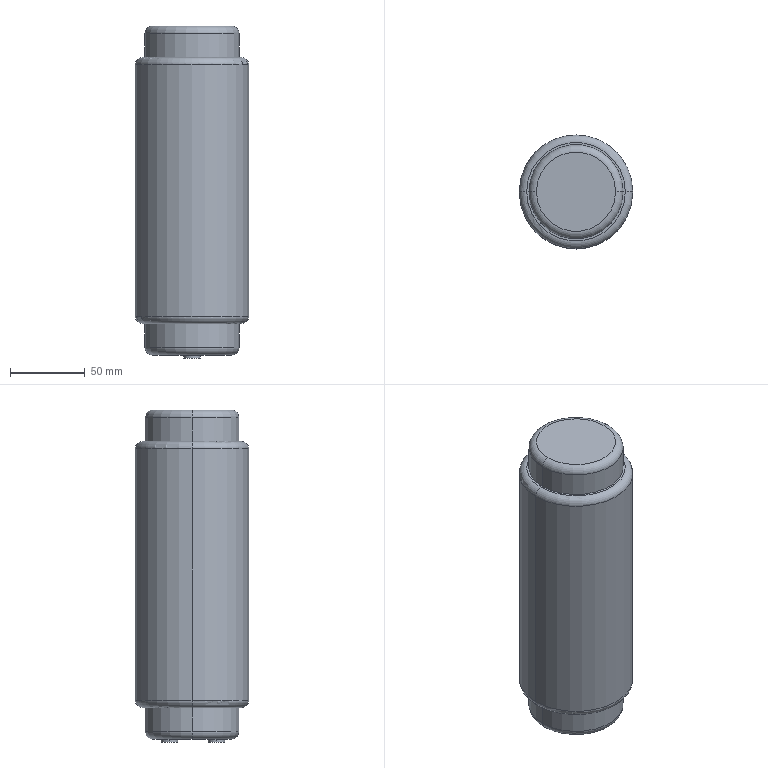Part | SolidWorks | features ICE 3, Extrusion 1, Fillet 1 | 1 solid | 24 faces | box 76 x 76 x 222 mm | volume 934259 mm3 | cylinder 10 | torus 8 | plane 6 | commonest cylinder face diameters 63 x4 10.958 x2 11.023 x2 76 x2
STEP:
#1=CARTESIAN_POINT('',(-5.511,-16.316,-112.));
#2=VERTEX_POINT('',#1);
#3=CARTESIAN_POINT('',(5.511,-16.316,-112.));
#4=VERTEX_POINT('',#3);
#5=CARTESIAN_POINT('',(0.,-16.316,-112.));
#6=DIRECTION('',(0.,0.,-1.));
#7=DIRECTION('',(-1.,0.,0.));
#8=AXIS2_PLACEMENT_3D('',#5,#6,#7);
#9=CIRCLE('',#8,5.511);
#10=EDGE_CURVE('',#2,#4,#9,.T.);
#11=ORIENTED_EDGE('',*,*,#10,.F.);
#12=CARTESIAN_POINT('',(-5.511,-16.316,-110.));
#13=VERTEX_POINT('',#12);
#14=CARTESIAN_POINT('',(-5.511,-16.316,-112.));
#15=DIRECTION('',(0.,0.,1.));
#16=VECTOR('',#15,1000.);
#17=LINE('',#14,#16);
#18=EDGE_CURVE('',#2,#13,#17,.T.);
#19=ORIENTED_EDGE('',*,*,#18,.T.);
#20=CARTESIAN_POINT('',(5.511,-16.316,-110.));
#21=VERTEX_POINT('',#20);
#22=CARTESIAN_POINT('',(0.,-16.316,-110.));
#23=DIRECTION('',(0.,0.,-1.));
#24=DIRECTION('',(1.,0.,0.));
#25=AXIS2_PLACEMENT_3D('',#22,#23,#24);
#26=CIRCLE('',#25,5.511);
#27=EDGE_CURVE('',#13,#21,#26,.T.);
#28=ORIENTED_EDGE('',*,*,#27,.T.);
#29=CARTESIAN_POINT('',(5.511,-16.316,-112.));
#30=DIRECTION('',(0.,0.,1.));
#31=VECTOR('',#30,1000.);
#32=LINE('',#29,#31);
#33=EDGE_CURVE('',#4,#21,#32,.T.);
#34=ORIENTED_EDGE('',*,*,#33,.F.);
#35=EDGE_LOOP('',(#11,#19,#28,#34));
#36=FACE_OUTER_BOUND('',#35,.T.);
#37=CARTESIAN_POINT('',(0.,-16.316,-112.));
#38=DIRECTION('',(0.,0.,1.));
#39=DIRECTION('',(1.,0.,0.));
#40=AXIS2_PLACEMENT_3D('',#37,#38,#39);
#41=CYLINDRICAL_SURFACE('',#40,5.511);
#42=ADVANCED_FACE('',(#36),#41,.T.);
#43=CARTESIAN_POINT('',(-5.479,15.014,-112.));
#44=VERTEX_POINT('',#43);
#45=CARTESIAN_POINT('',(5.479,15.014,-112.));
#46=VERTEX_POINT('',#45);
#47=CARTESIAN_POINT('',(0.,15.014,-112.));
#48=DIRECTION('',(0.,0.,-1.));
#49=DIRECTION('',(-1.,0.,0.));
#50=AXIS2_PLACEMENT_3D('',#47,#48,#49);
#51=CIRCLE('',#50,5.479);
#52=EDGE_CURVE('',#44,#46,#51,.T.);
#53=ORIENTED_EDGE('',*,*,#52,.F.);
#54=CARTESIAN_POINT('',(-5.479,15.014,-110.));
#55=VERTEX_POINT('',#54);
#56=CARTESIAN_POINT('',(-5.479,15.014,-112.));
#57=DIRECTION('',(0.,0.,1.));
#58=VECTOR('',#57,1000.);
#59=LINE('',#56,#58);
#60=EDGE_CURVE('',#44,#55,#59,.T.);
#61=ORIENTED_EDGE('',*,*,#60,.T.);
#62=CARTESIAN_POINT('',(5.479,15.014,-110.));
#63=VERTEX_POINT('',#62);
#64=CARTESIAN_POINT('',(0.,15.014,-110.));
#65=DIRECTION('',(0.,0.,-1.));
#66=DIRECTION('',(1.,0.,0.));
#67=AXIS2_PLACEMENT_3D('',#64,#65,#66);
#68=CIRCLE('',#67,5.479);
#69=EDGE_CURVE('',#55,#63,#68,.T.);
#70=ORIENTED_EDGE('',*,*,#69,.T.);
#71=CARTESIAN_POINT('',(5.479,15.014,-112.));
#72=DIRECTION('',(0.,0.,1.));
#73=VECTOR('',#72,1000.);
#74=LINE('',#71,#73);
#75=EDGE_CURVE('',#46,#63,#74,.T.);
#76=ORIENTED_EDGE('',*,*,#75,.F.);
#77=EDGE_LOOP('',(#53,#61,#70,#76));
#78=FACE_OUTER_BOUND('',#77,.T.);
#79=CARTESIAN_POINT('',(0.,15.014,-112.));
#80=DIRECTION('',(0.,0.,1.));
#81=DIRECTION('',(1.,0.,0.));
#82=AXIS2_PLACEMENT_3D('',#79,#80,#81);
#83=CYLINDRICAL_SURFACE('',#82,5.479);
#84=ADVANCED_FACE('',(#78),#83,.T.);
#85=CARTESIAN_POINT('',(-38.,0.,84.));
#86=VERTEX_POINT('',#85);
#87=CARTESIAN_POINT('',(38.,0.,84.));
#88=VERTEX_POINT('',#87);
#89=CARTESIAN_POINT('',(0.,0.,84.));
#90=DIRECTION('',(0.,0.,-1.));
#91=DIRECTION('',(1.,0.,0.));
#92=AXIS2_PLACEMENT_3D('',#89,#90,#91);
#93=CIRCLE('',#92,38.);
#94=EDGE_CURVE('',#86,#88,#93,.T.);
#95=ORIENTED_EDGE('',*,*,#94,.F.);
#96=CARTESIAN_POINT('',(-33.,0.,89.));
#97=VERTEX_POINT('',#96);
#98=CARTESIAN_POINT('',(-33.,0.,84.));
#99=DIRECTION('',(0.,1.,0.));
#100=DIRECTION('',(-1.,0.,0.));
#101=AXIS2_PLACEMENT_3D('',#98,#99,#100);
#102=CIRCLE('',#101,5.);
#103=EDGE_CURVE('',#86,#97,#102,.T.);
#104=ORIENTED_EDGE('',*,*,#103,.T.);
#105=CARTESIAN_POINT('',(33.,0.,89.));
#106=VERTEX_POINT('',#105);
#107=CARTESIAN_POINT('',(0.,0.,89.));
#108=DIRECTION('',(0.,0.,1.));
#109=DIRECTION('',(1.,0.,0.));
#110=AXIS2_PLACEMENT_3D('',#107,#108,#109);
#111=CIRCLE('',#110,33.);
#112=EDGE_CURVE('',#106,#97,#111,.T.);
#113=ORIENTED_EDGE('',*,*,#112,.F.);
#114=CARTESIAN_POINT('',(33.,0.,84.));
#115=DIRECTION('',(0.,-1.,0.));
#116=DIRECTION('',(0.,0.,-1.));
#117=AXIS2_PLACEMENT_3D('',#114,#115,#116);
#118=CIRCLE('',#117,5.);
#119=EDGE_CURVE('',#88,#106,#118,.T.);
#120=ORIENTED_EDGE('',*,*,#119,.F.);
#121=EDGE_LOOP('',(#95,#104,#113,#120));
#122=FACE_OUTER_BOUND('',#121,.T.);
#123=CARTESIAN_POINT('',(0.,0.,84.));
#124=DIRECTION('',(0.,0.,1.));
#125=DIRECTION('',(1.,0.,0.));
#126=AXIS2_PLACEMENT_3D('',#123,#124,#125);
#127=TOROIDAL_SURFACE('',#126,33.,5.);
#128=ADVANCED_FACE('',(#122),#127,.T.);
#129=CARTESIAN_POINT('',(38.,0.,-84.));
#130=VERTEX_POINT('',#129);
#131=CARTESIAN_POINT('',(-38.,0.,-84.));
#132=VERTEX_POINT('',#131);
#133=CARTESIAN_POINT('',(0.,0.,-84.));
#134=DIRECTION('',(0.,0.,1.));
#135=DIRECTION('',(-1.,0.,0.));
#136=AXIS2_PLACEMENT_3D('',#133,#134,#135);
#137=CIRCLE('',#136,38.);
#138=EDGE_CURVE('',#130,#132,#137,.T.);
#139=ORIENTED_EDGE('',*,*,#138,.F.);
#140=CARTESIAN_POINT('',(33.,0.,-89.));
#141=VERTEX_POINT('',#140);
#142=CARTESIAN_POINT('',(33.,0.,-84.));
#143=DIRECTION('',(0.,1.,0.));
#144=DIRECTION('',(-1.,0.,0.));
#145=AXIS2_PLACEMENT_3D('',#142,#143,#144);
#146=CIRCLE('',#145,5.);
#147=EDGE_CURVE('',#130,#141,#146,.T.);
#148=ORIENTED_EDGE('',*,*,#147,.T.);
#149=CARTESIAN_POINT('',(-33.,0.,-89.));
#150=VERTEX_POINT('',#149);
#151=CARTESIAN_POINT('',(0.,0.,-89.));
#152=DIRECTION('',(0.,0.,-1.));
#153=DIRECTION('',(-1.,0.,0.));
#154=AXIS2_PLACEMENT_3D('',#151,#152,#153);
#155=CIRCLE('',#154,33.);
#156=EDGE_CURVE('',#150,#141,#155,.T.);
#157=ORIENTED_EDGE('',*,*,#156,.F.);
#158=CARTESIAN_POINT('',(-33.,0.,-84.));
#159=DIRECTION('',(0.,-1.,0.));
#160=DIRECTION('',(0.,0.,-1.));
#161=AXIS2_PLACEMENT_3D('',#158,#159,#160);
#162=CIRCLE('',#161,5.);
#163=EDGE_CURVE('',#132,#150,#162,.T.);
#164=ORIENTED_EDGE('',*,*,#163,.F.);
#165=EDGE_LOOP('',(#139,#148,#157,#164));
#166=FACE_OUTER_BOUND('',#165,.T.);
#167=CARTESIAN_POINT('',(0.,0.,-84.));
#168=DIRECTION('',(0.,0.,-1.));
#169=DIRECTION('',(-1.,0.,0.));
#170=AXIS2_PLACEMENT_3D('',#167,#168,#169);
#171=TOROIDAL_SURFACE('',#170,33.,5.);
#172=ADVANCED_FACE('',(#166),#171,.T.);
#173=CARTESIAN_POINT('',(-26.5,0.,-110.));
#174=VERTEX_POINT('',#173);
#175=CARTESIAN_POINT('',(26.5,0.,-110.));
#176=VERTEX_POINT('',#175);
#177=CARTESIAN_POINT('',(0.,0.,-110.));
#178=DIRECTION('',(0.,0.,-1.));
#179=DIRECTION('',(1.,0.,0.));
#180=AXIS2_PLACEMENT_3D('',#177,#178,#179);
#181=CIRCLE('',#180,26.5);
#182=EDGE_CURVE('',#174,#176,#181,.T.);
#183=ORIENTED_EDGE('',*,*,#182,.F.);
#184=CARTESIAN_POINT('',(-31.5,0.,-105.));
#185=VERTEX_POINT('',#184);
#186=CARTESIAN_POINT('',(-26.5,0.,-105.));
#187=DIRECTION('',(0.,1.,0.));
#188=DIRECTION('',(-1.,0.,0.));
#189=AXIS2_PLACEMENT_3D('',#186,#187,#188);
#190=CIRCLE('',#189,5.);
#191=EDGE_CURVE('',#174,#185,#190,.T.);
#192=ORIENTED_EDGE('',*,*,#191,.T.);
#193=CARTESIAN_POINT('',(31.5,0.,-105.));
#194=VERTEX_POINT('',#193);
#195=CARTESIAN_POINT('',(0.,0.,-105.));
#196=DIRECTION('',(0.,0.,1.));
#197=DIRECTION('',(1.,0.,0.));
#198=AXIS2_PLACEMENT_3D('',#195,#196,#197);
#199=CIRCLE('',#198,31.5);
#200=EDGE_CURVE('',#194,#185,#199,.T.);
#201=ORIENTED_EDGE('',*,*,#200,.F.);
#202=CARTESIAN_POINT('',(26.5,0.,-105.));
#203=DIRECTION('',(0.,-1.,0.));
#204=DIRECTION('',(0.,0.,-1.));
#205=AXIS2_PLACEMENT_3D('',#202,#203,#204);
#206=CIRCLE('',#205,5.);
#207=EDGE_CURVE('',#176,#194,#206,.T.);
#208=ORIENTED_EDGE('',*,*,#207,.F.);
#209=EDGE_LOOP('',(#183,#192,#201,#208));
#210=FACE_OUTER_BOUND('',#209,.T.);
#211=CARTESIAN_POINT('',(0.,0.,-105.));
#212=DIRECTION('',(0.,0.,1.));
#213=DIRECTION('',(1.,0.,0.));
#214=AXIS2_PLACEMENT_3D('',#211,#212,#213);
#215=TOROIDAL_SURFACE('',#214,26.5,5.);
#216=ADVANCED_FACE('',(#210),#215,.T.);
#217=CARTESIAN_POINT('',(-31.5,0.,105.));
#218=VERTEX_POINT('',#217);
#219=CARTESIAN_POINT('',(31.5,0.,105.));
#220=VERTEX_POINT('',#219);
#221=CARTESIAN_POINT('',(0.,0.,105.));
#222=DIRECTION('',(0.,0.,-1.));
#223=DIRECTION('',(1.,0.,0.));
#224=AXIS2_PLACEMENT_3D('',#221,#222,#223);
#225=CIRCLE('',#224,31.5);
#226=EDGE_CURVE('',#218,#220,#225,.T.);
#227=ORIENTED_EDGE('',*,*,#226,.F.);
#228=CARTESIAN_POINT('',(-26.5,0.,110.));
#229=VERTEX_POINT('',#228);
#230=CARTESIAN_POINT('',(-26.5,0.,105.));
#231=DIRECTION('',(0.,1.,0.));
#232=DIRECTION('',(-1.,0.,0.));
#233=AXIS2_PLACEMENT_3D('',#230,#231,#232);
#234=CIRCLE('',#233,5.);
#235=EDGE_CURVE('',#218,#229,#234,.T.);
#236=ORIENTED_EDGE('',*,*,#235,.T.);
#237=CARTESIAN_POINT('',(26.5,0.,110.));
#238=VERTEX_POINT('',#237);
#239=CARTESIAN_POINT('',(0.,0.,110.));
#240=DIRECTION('',(0.,0.,1.));
#241=DIRECTION('',(1.,0.,0.));
#242=AXIS2_PLACEMENT_3D('',#239,#240,#241);
#243=CIRCLE('',#242,26.5);
#244=EDGE_CURVE('',#238,#229,#243,.T.);
#245=ORIENTED_EDGE('',*,*,#244,.F.);
#246=CARTESIAN_POINT('',(26.5,0.,105.));
#247=DIRECTION('',(0.,-1.,0.));
#248=DIRECTION('',(0.,0.,-1.));
#249=AXIS2_PLACEMENT_3D('',#246,#247,#248);
#250=CIRCLE('',#249,5.);
#251=EDGE_CURVE('',#220,#238,#250,.T.);
#252=ORIENTED_EDGE('',*,*,#251,.F.);
#253=EDGE_LOOP('',(#227,#236,#245,#252));
#254=FACE_OUTER_BOUND('',#253,.T.);
#255=CARTESIAN_POINT('',(0.,0.,105.));
#256=DIRECTION('',(0.,0.,1.));
#257=DIRECTION('',(1.,0.,0.));
#258=AXIS2_PLACEMENT_3D('',#255,#256,#257);
#259=TOROIDAL_SURFACE('',#258,26.5,5.);
#260=ADVANCED_FACE('',(#254),#259,.T.);
#261=CARTESIAN_POINT('',(-31.5,0.,-89.));
#262=VERTEX_POINT('',#261);
#263=CARTESIAN_POINT('',(31.5,0.,-89.));
#264=VERTEX_POINT('',#263);
#265=CARTESIAN_POINT('',(0.,0.,-89.));
#266=DIRECTION('',(0.,0.,-1.));
#267=DIRECTION('',(-1.,0.,0.));
#268=AXIS2_PLACEMENT_3D('',#265,#266,#267);
#269=CIRCLE('',#268,31.5);
#270=EDGE_CURVE('',#262,#264,#269,.T.);
#271=ORIENTED_EDGE('',*,*,#270,.T.);
#272=CARTESIAN_POINT('',(31.5,0.,-89.));
#273=DIRECTION('',(0.,0.,-1.));
#274=VECTOR('',#273,1000.);
#275=LINE('',#272,#274);
#276=EDGE_CURVE('',#264,#194,#275,.T.);
#277=ORIENTED_EDGE('',*,*,#276,.T.);
#278=ORIENTED_EDGE('',*,*,#200,.T.);
#279=CARTESIAN_POINT('',(-31.5,0.,-89.));
#280=DIRECTION('',(0.,0.,-1.));
#281=VECTOR('',#280,1000.);
#282=LINE('',#279,#281);
#283=EDGE_CURVE('',#262,#185,#282,.T.);
#284=ORIENTED_EDGE('',*,*,#283,.F.);
#285=EDGE_LOOP('',(#271,#277,#278,#284));
#286=FACE_OUTER_BOUND('',#285,.T.);
#287=CARTESIAN_POINT('',(0.,0.,-89.));
#288=DIRECTION('',(0.,0.,-1.));
#289=DIRECTION('',(-1.,0.,0.));
#290=AXIS2_PLACEMENT_3D('',#287,#288,#289);
#291=CYLINDRICAL_SURFACE('',#290,31.5);
#292=ADVANCED_FACE('',(#286),#291,.T.);
#293=CARTESIAN_POINT('',(31.5,0.,89.));
#294=VERTEX_POINT('',#293);
#295=CARTESIAN_POINT('',(-31.5,0.,89.));
#296=VERTEX_POINT('',#295);
#297=CARTESIAN_POINT('',(0.,0.,89.));
#298=DIRECTION('',(0.,0.,1.));
#299=DIRECTION('',(1.,0.,0.));
#300=AXIS2_PLACEMENT_3D('',#297,#298,#299);
#301=CIRCLE('',#300,31.5);
#302=EDGE_CURVE('',#294,#296,#301,.T.);
#303=ORIENTED_EDGE('',*,*,#302,.T.);
#304=CARTESIAN_POINT('',(-31.5,0.,89.));
#305=DIRECTION('',(0.,0.,1.));
#306=VECTOR('',#305,1000.);
#307=LINE('',#304,#306);
#308=EDGE_CURVE('',#296,#218,#307,.T.);
#309=ORIENTED_EDGE('',*,*,#308,.T.);
#310=ORIENTED_EDGE('',*,*,#226,.T.);
#311=CARTESIAN_POINT('',(31.5,0.,89.));
#312=DIRECTION('',(0.,0.,1.));
#313=VECTOR('',#312,1000.);
#314=LINE('',#311,#313);
#315=EDGE_CURVE('',#294,#220,#314,.T.);
#316=ORIENTED_EDGE('',*,*,#315,.F.);
#317=EDGE_LOOP('',(#303,#309,#310,#316));
#318=FACE_OUTER_BOUND('',#317,.T.);
#319=CARTESIAN_POINT('',(0.,0.,89.));
#320=DIRECTION('',(0.,0.,1.));
#321=DIRECTION('',(1.,0.,0.));
#322=AXIS2_PLACEMENT_3D('',#319,#320,#321);
#323=CYLINDRICAL_SURFACE('',#322,31.5);
#324=ADVANCED_FACE('',(#318),#323,.T.);
#325=ORIENTED_EDGE('',*,*,#94,.T.);
#326=CARTESIAN_POINT('',(38.,0.,110.));
#327=DIRECTION('',(0.,0.,-1.));
#328=VECTOR('',#327,1000.);
#329=LINE('',#326,#328);
#330=EDGE_CURVE('',#88,#130,#329,.T.);
#331=ORIENTED_EDGE('',*,*,#330,.T.);
#332=ORIENTED_EDGE('',*,*,#138,.T.);
#333=CARTESIAN_POINT('',(-38.,0.,110.));
#334=DIRECTION('',(0.,0.,-1.));
#335=VECTOR('',#334,1000.);
#336=LINE('',#333,#335);
#337=EDGE_CURVE('',#86,#132,#336,.T.);
#338=ORIENTED_EDGE('',*,*,#337,.F.);
#339=EDGE_LOOP('',(#325,#331,#332,#338));
#340=FACE_OUTER_BOUND('',#339,.T.);
#341=CARTESIAN_POINT('',(0.,0.,110.));
#342=DIRECTION('',(0.,0.,-1.));
#343=DIRECTION('',(-1.,0.,0.));
#344=AXIS2_PLACEMENT_3D('',#341,#342,#343);
#345=CYLINDRICAL_SURFACE('',#344,38.);
#346=ADVANCED_FACE('',(#340),#345,.T.);
#347=ORIENTED_EDGE('',*,*,#330,.F.);
#348=CARTESIAN_POINT('',(0.,0.,84.));
#349=DIRECTION('',(0.,0.,-1.));
#350=DIRECTION('',(1.,0.,0.));
#351=AXIS2_PLACEMENT_3D('',#348,#349,#350);
#352=CIRCLE('',#351,38.);
#353=EDGE_CURVE('',#88,#86,#352,.T.);
#354=ORIENTED_EDGE('',*,*,#353,.T.);
#355=ORIENTED_EDGE('',*,*,#337,.T.);
#356=CARTESIAN_POINT('',(0.,0.,-84.));
#357=DIRECTION('',(0.,0.,1.));
#358=DIRECTION('',(-1.,0.,0.));
#359=AXIS2_PLACEMENT_3D('',#356,#357,#358);
#360=CIRCLE('',#359,38.);
#361=EDGE_CURVE('',#132,#130,#360,.T.);
#362=ORIENTED_EDGE('',*,*,#361,.T.);
#363=EDGE_LOOP('',(#347,#354,#355,#362));
#364=FACE_OUTER_BOUND('',#363,.T.);
#365=CARTESIAN_POINT('',(0.,0.,110.));
#366=DIRECTION('',(0.,0.,-1.));
#367=DIRECTION('',(-1.,0.,0.));
#368=AXIS2_PLACEMENT_3D('',#365,#366,#367);
#369=CYLINDRICAL_SURFACE('',#368,38.);
#370=ADVANCED_FACE('',(#364),#369,.T.);
#371=ORIENTED_EDGE('',*,*,#112,.T.);
#372=CARTESIAN_POINT('',(0.,0.,89.));
#373=DIRECTION('',(0.,0.,1.));
#374=DIRECTION('',(1.,0.,0.));
#375=AXIS2_PLACEMENT_3D('',#372,#373,#374);
#376=CIRCLE('',#375,33.);
#377=EDGE_CURVE('',#97,#106,#376,.T.);
#378=ORIENTED_EDGE('',*,*,#377,.T.);
#379=EDGE_LOOP('',(#371,#378));
#380=FACE_OUTER_BOUND('',#379,.T.);
#381=ORIENTED_EDGE('',*,*,#302,.F.);
#382=CARTESIAN_POINT('',(0.,0.,89.));
#383=DIRECTION('',(0.,0.,1.));
#384=DIRECTION('',(1.,0.,0.));
#385=AXIS2_PLACEMENT_3D('',#382,#383,#384);
#386=CIRCLE('',#385,31.5);
#387=EDGE_CURVE('',#296,#294,#386,.T.);
#388=ORIENTED_EDGE('',*,*,#387,.F.);
#389=EDGE_LOOP('',(#381,#388));
#390=FACE_BOUND('',#389,.T.);
#391=CARTESIAN_POINT('',(0.,0.,89.));
#392=DIRECTION('',(0.,0.,1.));
#393=DIRECTION('',(1.,0.,0.));
#394=AXIS2_PLACEMENT_3D('',#391,#392,#393);
#395=PLANE('',#394);
#396=ADVANCED_FACE('',(#380,#390),#395,.T.);
#397=ORIENTED_EDGE('',*,*,#308,.F.);
#398=ORIENTED_EDGE('',*,*,#387,.T.);
#399=ORIENTED_EDGE('',*,*,#315,.T.);
#400=CARTESIAN_POINT('',(0.,0.,105.));
#401=DIRECTION('',(0.,0.,-1.));
#402=DIRECTION('',(1.,0.,0.));
#403=AXIS2_PLACEMENT_3D('',#400,#401,#402);
#404=CIRCLE('',#403,31.5);
#405=EDGE_CURVE('',#220,#218,#404,.T.);
#406=ORIENTED_EDGE('',*,*,#405,.T.);
#407=EDGE_LOOP('',(#397,#398,#399,#406));
#408=FACE_OUTER_BOUND('',#407,.T.);
#409=CARTESIAN_POINT('',(0.,0.,89.));
#410=DIRECTION('',(0.,0.,1.));
#411=DIRECTION('',(1.,0.,0.));
#412=AXIS2_PLACEMENT_3D('',#409,#410,#411);
#413=CYLINDRICAL_SURFACE('',#412,31.5);
#414=ADVANCED_FACE('',(#408),#413,.T.);
#415=ORIENTED_EDGE('',*,*,#244,.T.);
#416=CARTESIAN_POINT('',(0.,0.,110.));
#417=DIRECTION('',(0.,0.,1.));
#418=DIRECTION('',(1.,0.,0.));
#419=AXIS2_PLACEMENT_3D('',#416,#417,#418);
#420=CIRCLE('',#419,26.5);
#421=EDGE_CURVE('',#229,#238,#420,.T.);
#422=ORIENTED_EDGE('',*,*,#421,.T.);
#423=EDGE_LOOP('',(#415,#422));
#424=FACE_OUTER_BOUND('',#423,.T.);
#425=CARTESIAN_POINT('',(0.,0.,110.));
#426=DIRECTION('',(0.,0.,1.));
#427=DIRECTION('',(1.,0.,0.));
#428=AXIS2_PLACEMENT_3D('',#425,#426,#427);
#429=PLANE('',#428);
#430=ADVANCED_FACE('',(#424),#429,.T.);
#431=ORIENTED_EDGE('',*,*,#156,.T.);
#432=CARTESIAN_POINT('',(0.,0.,-89.));
#433=DIRECTION('',(0.,0.,-1.));
#434=DIRECTION('',(-1.,0.,0.));
#435=AXIS2_PLACEMENT_3D('',#432,#433,#434);
#436=CIRCLE('',#435,33.);
#437=EDGE_CURVE('',#141,#150,#436,.T.);
#438=ORIENTED_EDGE('',*,*,#437,.T.);
#439=EDGE_LOOP('',(#431,#438));
#440=FACE_OUTER_BOUND('',#439,.T.);
#441=ORIENTED_EDGE('',*,*,#270,.F.);
#442=CARTESIAN_POINT('',(0.,0.,-89.));
#443=DIRECTION('',(0.,0.,-1.));
#444=DIRECTION('',(-1.,0.,0.));
#445=AXIS2_PLACEMENT_3D('',#442,#443,#444);
#446=CIRCLE('',#445,31.5);
#447=EDGE_CURVE('',#264,#262,#446,.T.);
#448=ORIENTED_EDGE('',*,*,#447,.F.);
#449=EDGE_LOOP('',(#441,#448));
#450=FACE_BOUND('',#449,.T.);
#451=CARTESIAN_POINT('',(0.,0.,-89.));
#452=DIRECTION('',(0.,0.,-1.));
#453=DIRECTION('',(-1.,0.,0.));
#454=AXIS2_PLACEMENT_3D('',#451,#452,#453);
#455=PLANE('',#454);
#456=ADVANCED_FACE('',(#440,#450),#455,.T.);
#457=ORIENTED_EDGE('',*,*,#276,.F.);
#458=ORIENTED_EDGE('',*,*,#447,.T.);
#459=ORIENTED_EDGE('',*,*,#283,.T.);
#460=CARTESIAN_POINT('',(0.,0.,-105.));
#461=DIRECTION('',(0.,0.,1.));
#462=DIRECTION('',(1.,0.,0.));
#463=AXIS2_PLACEMENT_3D('',#460,#461,#462);
#464=CIRCLE('',#463,31.5);
#465=EDGE_CURVE('',#185,#194,#464,.T.);
#466=ORIENTED_EDGE('',*,*,#465,.T.);
#467=EDGE_LOOP('',(#457,#458,#459,#466));
#468=FACE_OUTER_BOUND('',#467,.T.);
#469=CARTESIAN_POINT('',(0.,0.,-89.));
#470=DIRECTION('',(0.,0.,-1.));
#471=DIRECTION('',(-1.,0.,0.));
#472=AXIS2_PLACEMENT_3D('',#469,#470,#471);
#473=CYLINDRICAL_SURFACE('',#472,31.5);
#474=ADVANCED_FACE('',(#468),#473,.T.);
#475=CARTESIAN_POINT('',(0.,-16.316,-110.));
#476=DIRECTION('',(0.,0.,-1.));
#477=DIRECTION('',(1.,0.,0.));
#478=AXIS2_PLACEMENT_3D('',#475,#476,#477);
#479=CIRCLE('',#478,5.511);
#480=EDGE_CURVE('',#21,#13,#479,.T.);
#481=ORIENTED_EDGE('',*,*,#480,.F.);
#482=ORIENTED_EDGE('',*,*,#27,.F.);
#483=EDGE_LOOP('',(#481,#482));
#484=FACE_BOUND('',#483,.T.);
#485=CARTESIAN_POINT('',(0.,15.014,-110.));
#486=DIRECTION('',(0.,0.,-1.));
#487=DIRECTION('',(1.,0.,0.));
#488=AXIS2_PLACEMENT_3D('',#485,#486,#487);
#489=CIRCLE('',#488,5.479);
#490=EDGE_CURVE('',#63,#55,#489,.T.);
#491=ORIENTED_EDGE('',*,*,#490,.F.);
#492=ORIENTED_EDGE('',*,*,#69,.F.);
#493=EDGE_LOOP('',(#491,#492));
#494=FACE_BOUND('',#493,.T.);
#495=CARTESIAN_POINT('',(0.,0.,-110.));
#496=DIRECTION('',(0.,0.,-1.));
#497=DIRECTION('',(1.,0.,0.));
#498=AXIS2_PLACEMENT_3D('',#495,#496,#497);
#499=CIRCLE('',#498,26.5);
#500=EDGE_CURVE('',#176,#174,#499,.T.);
#501=ORIENTED_EDGE('',*,*,#500,.T.);
#502=ORIENTED_EDGE('',*,*,#182,.T.);
#503=EDGE_LOOP('',(#501,#502));
#504=FACE_OUTER_BOUND('',#503,.T.);
#505=CARTESIAN_POINT('',(0.,0.,-110.));
#506=DIRECTION('',(0.,0.,1.));
#507=DIRECTION('',(1.,0.,0.));
#508=AXIS2_PLACEMENT_3D('',#505,#506,#507);
#509=PLANE('',#508);
#510=ADVANCED_FACE('',(#484,#494,#504),#509,.F.);
#511=ORIENTED_EDGE('',*,*,#235,.F.);
#512=ORIENTED_EDGE('',*,*,#405,.F.);
#513=ORIENTED_EDGE('',*,*,#251,.T.);
#514=ORIENTED_EDGE('',*,*,#421,.F.);
#515=EDGE_LOOP('',(#511,#512,#513,#514));
#516=FACE_OUTER_BOUND('',#515,.T.);
#517=CARTESIAN_POINT('',(0.,0.,105.));
#518=DIRECTION('',(0.,0.,1.));
#519=DIRECTION('',(1.,0.,0.));
#520=AXIS2_PLACEMENT_3D('',#517,#518,#519);
#521=TOROIDAL_SURFACE('',#520,26.5,5.);
#522=ADVANCED_FACE('',(#516),#521,.T.);
#523=ORIENTED_EDGE('',*,*,#191,.F.);
#524=ORIENTED_EDGE('',*,*,#500,.F.);
#525=ORIENTED_EDGE('',*,*,#207,.T.);
#526=ORIENTED_EDGE('',*,*,#465,.F.);
#527=EDGE_LOOP('',(#523,#524,#525,#526));
#528=FACE_OUTER_BOUND('',#527,.T.);
#529=CARTESIAN_POINT('',(0.,0.,-105.));
#530=DIRECTION('',(0.,0.,1.));
#531=DIRECTION('',(1.,0.,0.));
#532=AXIS2_PLACEMENT_3D('',#529,#530,#531);
#533=TOROIDAL_SURFACE('',#532,26.5,5.);
#534=ADVANCED_FACE('',(#528),#533,.T.);
#535=ORIENTED_EDGE('',*,*,#147,.F.);
#536=ORIENTED_EDGE('',*,*,#361,.F.);
#537=ORIENTED_EDGE('',*,*,#163,.T.);
#538=ORIENTED_EDGE('',*,*,#437,.F.);
#539=EDGE_LOOP('',(#535,#536,#537,#538));
#540=FACE_OUTER_BOUND('',#539,.T.);
#541=CARTESIAN_POINT('',(0.,0.,-84.));
#542=DIRECTION('',(0.,0.,-1.));
#543=DIRECTION('',(-1.,0.,0.));
#544=AXIS2_PLACEMENT_3D('',#541,#542,#543);
#545=TOROIDAL_SURFACE('',#544,33.,5.);
#546=ADVANCED_FACE('',(#540),#545,.T.);
#547=ORIENTED_EDGE('',*,*,#103,.F.);
#548=ORIENTED_EDGE('',*,*,#353,.F.);
#549=ORIENTED_EDGE('',*,*,#119,.T.);
#550=ORIENTED_EDGE('',*,*,#377,.F.);
#551=EDGE_LOOP('',(#547,#548,#549,#550));
#552=FACE_OUTER_BOUND('',#551,.T.);
#553=CARTESIAN_POINT('',(0.,0.,84.));
#554=DIRECTION('',(0.,0.,1.));
#555=DIRECTION('',(1.,0.,0.));
#556=AXIS2_PLACEMENT_3D('',#553,#554,#555);
#557=TOROIDAL_SURFACE('',#556,33.,5.);
#558=ADVANCED_FACE('',(#552),#557,.T.);
#559=ORIENTED_EDGE('',*,*,#60,.F.);
#560=CARTESIAN_POINT('',(0.,15.014,-112.));
#561=DIRECTION('',(0.,0.,-1.));
#562=DIRECTION('',(-1.,0.,0.));
#563=AXIS2_PLACEMENT_3D('',#560,#561,#562);
#564=CIRCLE('',#563,5.479);
#565=EDGE_CURVE('',#46,#44,#564,.T.);
#566=ORIENTED_EDGE('',*,*,#565,.F.);
#567=ORIENTED_EDGE('',*,*,#75,.T.);
#568=ORIENTED_EDGE('',*,*,#490,.T.);
#569=EDGE_LOOP('',(#559,#566,#567,#568));
#570=FACE_OUTER_BOUND('',#569,.T.);
#571=CARTESIAN_POINT('',(0.,15.014,-112.));
#572=DIRECTION('',(0.,0.,1.));
#573=DIRECTION('',(1.,0.,0.));
#574=AXIS2_PLACEMENT_3D('',#571,#572,#573);
#575=CYLINDRICAL_SURFACE('',#574,5.479);
#576=ADVANCED_FACE('',(#570),#575,.T.);
#577=ORIENTED_EDGE('',*,*,#565,.T.);
#578=ORIENTED_EDGE('',*,*,#52,.T.);
#579=EDGE_LOOP('',(#577,#578));
#580=FACE_OUTER_BOUND('',#579,.T.);
#581=CARTESIAN_POINT('',(0.,15.014,-112.));
#582=DIRECTION('',(0.,0.,-1.));
#583=DIRECTION('',(-1.,0.,0.));
#584=AXIS2_PLACEMENT_3D('',#581,#582,#583);
#585=PLANE('',#584);
#586=ADVANCED_FACE('',(#580),#585,.T.);
#587=ORIENTED_EDGE('',*,*,#18,.F.);
#588=CARTESIAN_POINT('',(0.,-16.316,-112.));
#589=DIRECTION('',(0.,0.,-1.));
#590=DIRECTION('',(-1.,0.,0.));
#591=AXIS2_PLACEMENT_3D('',#588,#589,#590);
#592=CIRCLE('',#591,5.511);
#593=EDGE_CURVE('',#4,#2,#592,.T.);
#594=ORIENTED_EDGE('',*,*,#593,.F.);
#595=ORIENTED_EDGE('',*,*,#33,.T.);
#596=ORIENTED_EDGE('',*,*,#480,.T.);
#597=EDGE_LOOP('',(#587,#594,#595,#596));
#598=FACE_OUTER_BOUND('',#597,.T.);
#599=CARTESIAN_POINT('',(0.,-16.316,-112.));
#600=DIRECTION('',(0.,0.,1.));
#601=DIRECTION('',(1.,0.,0.));
#602=AXIS2_PLACEMENT_3D('',#599,#600,#601);
#603=CYLINDRICAL_SURFACE('',#602,5.511);
#604=ADVANCED_FACE('',(#598),#603,.T.);
#605=ORIENTED_EDGE('',*,*,#593,.T.);
#606=ORIENTED_EDGE('',*,*,#10,.T.);
#607=EDGE_LOOP('',(#605,#606));
#608=FACE_OUTER_BOUND('',#607,.T.);
#609=CARTESIAN_POINT('',(0.,-16.316,-112.));
#610=DIRECTION('',(0.,0.,-1.));
#611=DIRECTION('',(-1.,0.,0.));
#612=AXIS2_PLACEMENT_3D('',#609,#610,#611);
#613=PLANE('',#612);
#614=ADVANCED_FACE('',(#608),#613,.T.);
#615=CLOSED_SHELL('',(#42,#84,#128,#172,#216,#260,#292,#324,#346,#370,#396,#414,#430,#456,#474,#510,#522,#534,#546,#558,#576,#586,#604,#614));
#616=MANIFOLD_SOLID_BREP('',#615);
#617=CARTESIAN_POINT('',(0.,0.,0.));
#618=DIRECTION('',(0.,0.,1.));
#619=DIRECTION('',(1.,0.,0.));
#620=AXIS2_PLACEMENT_3D('',#617,#618,#619);
#621=(LENGTH_UNIT()NAMED_UNIT(*)SI_UNIT(.MILLI.,.METRE.));
#622=UNCERTAINTY_MEASURE_WITH_UNIT(LENGTH_MEASURE(0.00001),#621,'','');
#623=(NAMED_UNIT(*)PLANE_ANGLE_UNIT()SI_UNIT($,.RADIAN.));
#624=(NAMED_UNIT(*)SI_UNIT($,.STERADIAN.)SOLID_ANGLE_UNIT());
#625=(GEOMETRIC_REPRESENTATION_CONTEXT(3)GLOBAL_UNCERTAINTY_ASSIGNED_CONTEXT((#622))GLOBAL_UNIT_ASSIGNED_CONTEXT((#621,#623,#624))REPRESENTATION_CONTEXT('',''));
#626=ADVANCED_BREP_SHAPE_REPRESENTATION('',(#616,#620),#625);